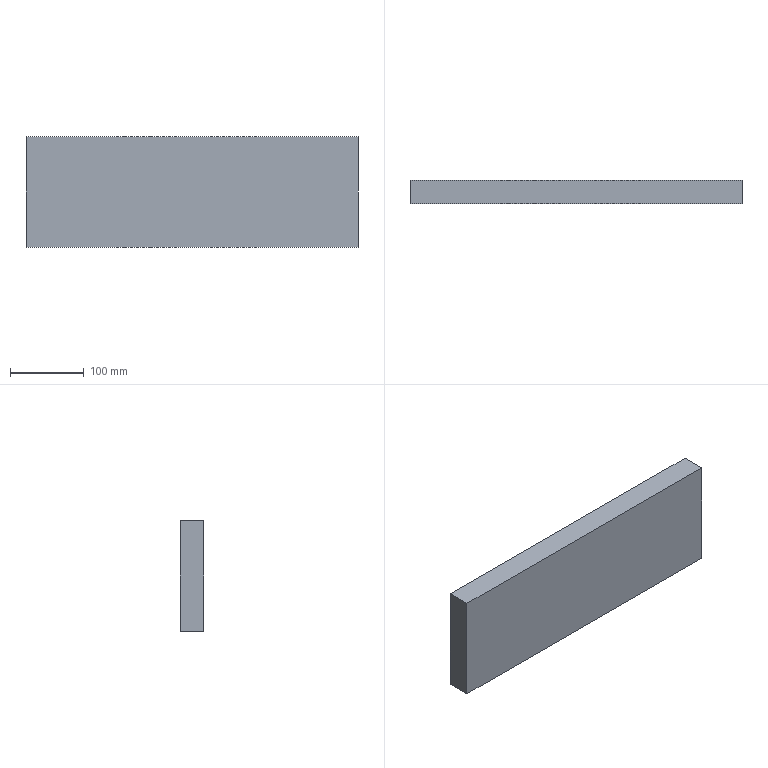Part | NX | 1 solid | 6 faces | box 450 x 32 x 150 mm | volume 2160000 mm3 | plane 6
STEP:
#1=CARTESIAN_POINT('',(225.,0.,75.));
#2=VERTEX_POINT('',#1);
#3=CARTESIAN_POINT('',(225.,0.,-75.));
#4=VERTEX_POINT('',#3);
#5=CARTESIAN_POINT('',(225.,0.,75.));
#6=DIRECTION('',(0.,0.,-1.));
#7=VECTOR('',#6,1000.);
#8=LINE('',#5,#7);
#9=EDGE_CURVE('',#2,#4,#8,.T.);
#10=ORIENTED_EDGE('',*,*,#9,.T.);
#11=CARTESIAN_POINT('',(225.,32.,-75.));
#12=VERTEX_POINT('',#11);
#13=CARTESIAN_POINT('',(225.,32.,-75.));
#14=DIRECTION('',(0.,-1.,0.));
#15=VECTOR('',#14,1000.);
#16=LINE('',#13,#15);
#17=EDGE_CURVE('',#12,#4,#16,.T.);
#18=ORIENTED_EDGE('',*,*,#17,.F.);
#19=CARTESIAN_POINT('',(225.,32.,75.));
#20=VERTEX_POINT('',#19);
#21=CARTESIAN_POINT('',(225.,32.,75.));
#22=DIRECTION('',(0.,0.,-1.));
#23=VECTOR('',#22,1000.);
#24=LINE('',#21,#23);
#25=EDGE_CURVE('',#20,#12,#24,.T.);
#26=ORIENTED_EDGE('',*,*,#25,.F.);
#27=CARTESIAN_POINT('',(225.,32.,75.));
#28=DIRECTION('',(0.,-1.,0.));
#29=VECTOR('',#28,1000.);
#30=LINE('',#27,#29);
#31=EDGE_CURVE('',#20,#2,#30,.T.);
#32=ORIENTED_EDGE('',*,*,#31,.T.);
#33=EDGE_LOOP('',(#10,#18,#26,#32));
#34=FACE_BOUND('',#33,.T.);
#35=CARTESIAN_POINT('',(225.,32.,75.));
#36=DIRECTION('',(-1.,0.,0.));
#37=DIRECTION('',(0.,0.,1.));
#38=AXIS2_PLACEMENT_3D('',#35,#36,#37);
#39=PLANE('',#38);
#40=ADVANCED_FACE('',(#34),#39,.F.);
#41=CARTESIAN_POINT('',(-225.,0.,-75.));
#42=VERTEX_POINT('',#41);
#43=CARTESIAN_POINT('',(-225.,0.,-75.));
#44=DIRECTION('',(-1.,0.,0.));
#45=VECTOR('',#44,1000.);
#46=LINE('',#43,#45);
#47=EDGE_CURVE('',#4,#42,#46,.T.);
#48=ORIENTED_EDGE('',*,*,#47,.T.);
#49=CARTESIAN_POINT('',(-225.,32.,-75.));
#50=VERTEX_POINT('',#49);
#51=CARTESIAN_POINT('',(-225.,32.,-75.));
#52=DIRECTION('',(0.,-1.,0.));
#53=VECTOR('',#52,1000.);
#54=LINE('',#51,#53);
#55=EDGE_CURVE('',#50,#42,#54,.T.);
#56=ORIENTED_EDGE('',*,*,#55,.F.);
#57=CARTESIAN_POINT('',(-225.,32.,-75.));
#58=DIRECTION('',(-1.,0.,0.));
#59=VECTOR('',#58,1000.);
#60=LINE('',#57,#59);
#61=EDGE_CURVE('',#12,#50,#60,.T.);
#62=ORIENTED_EDGE('',*,*,#61,.F.);
#63=ORIENTED_EDGE('',*,*,#17,.T.);
#64=EDGE_LOOP('',(#48,#56,#62,#63));
#65=FACE_BOUND('',#64,.T.);
#66=CARTESIAN_POINT('',(-225.,32.,-75.));
#67=DIRECTION('',(0.,0.,1.));
#68=DIRECTION('',(1.,0.,0.));
#69=AXIS2_PLACEMENT_3D('',#66,#67,#68);
#70=PLANE('',#69);
#71=ADVANCED_FACE('',(#65),#70,.F.);
#72=CARTESIAN_POINT('',(-225.,0.,75.));
#73=VERTEX_POINT('',#72);
#74=CARTESIAN_POINT('',(-225.,0.,75.));
#75=DIRECTION('',(0.,0.,1.));
#76=VECTOR('',#75,1000.);
#77=LINE('',#74,#76);
#78=EDGE_CURVE('',#42,#73,#77,.T.);
#79=ORIENTED_EDGE('',*,*,#78,.T.);
#80=CARTESIAN_POINT('',(-225.,32.,75.));
#81=VERTEX_POINT('',#80);
#82=CARTESIAN_POINT('',(-225.,32.,75.));
#83=DIRECTION('',(0.,-1.,0.));
#84=VECTOR('',#83,1000.);
#85=LINE('',#82,#84);
#86=EDGE_CURVE('',#81,#73,#85,.T.);
#87=ORIENTED_EDGE('',*,*,#86,.F.);
#88=CARTESIAN_POINT('',(-225.,32.,75.));
#89=DIRECTION('',(0.,0.,1.));
#90=VECTOR('',#89,1000.);
#91=LINE('',#88,#90);
#92=EDGE_CURVE('',#50,#81,#91,.T.);
#93=ORIENTED_EDGE('',*,*,#92,.F.);
#94=ORIENTED_EDGE('',*,*,#55,.T.);
#95=EDGE_LOOP('',(#79,#87,#93,#94));
#96=FACE_BOUND('',#95,.T.);
#97=CARTESIAN_POINT('',(-225.,32.,75.));
#98=DIRECTION('',(1.,0.,0.));
#99=DIRECTION('',(0.,0.,-1.));
#100=AXIS2_PLACEMENT_3D('',#97,#98,#99);
#101=PLANE('',#100);
#102=ADVANCED_FACE('',(#96),#101,.F.);
#103=CARTESIAN_POINT('',(-225.,0.,75.));
#104=DIRECTION('',(1.,0.,0.));
#105=VECTOR('',#104,1000.);
#106=LINE('',#103,#105);
#107=EDGE_CURVE('',#73,#2,#106,.T.);
#108=ORIENTED_EDGE('',*,*,#107,.T.);
#109=ORIENTED_EDGE('',*,*,#31,.F.);
#110=CARTESIAN_POINT('',(-225.,32.,75.));
#111=DIRECTION('',(1.,0.,0.));
#112=VECTOR('',#111,1000.);
#113=LINE('',#110,#112);
#114=EDGE_CURVE('',#81,#20,#113,.T.);
#115=ORIENTED_EDGE('',*,*,#114,.F.);
#116=ORIENTED_EDGE('',*,*,#86,.T.);
#117=EDGE_LOOP('',(#108,#109,#115,#116));
#118=FACE_BOUND('',#117,.T.);
#119=CARTESIAN_POINT('',(-225.,32.,75.));
#120=DIRECTION('',(0.,0.,-1.));
#121=DIRECTION('',(-1.,0.,0.));
#122=AXIS2_PLACEMENT_3D('',#119,#120,#121);
#123=PLANE('',#122);
#124=ADVANCED_FACE('',(#118),#123,.F.);
#125=ORIENTED_EDGE('',*,*,#25,.T.);
#126=ORIENTED_EDGE('',*,*,#61,.T.);
#127=ORIENTED_EDGE('',*,*,#92,.T.);
#128=ORIENTED_EDGE('',*,*,#114,.T.);
#129=EDGE_LOOP('',(#125,#126,#127,#128));
#130=FACE_BOUND('',#129,.T.);
#131=CARTESIAN_POINT('',(0.,32.,0.));
#132=DIRECTION('',(0.,-1.,0.));
#133=DIRECTION('',(0.,0.,-1.));
#134=AXIS2_PLACEMENT_3D('',#131,#132,#133);
#135=PLANE('',#134);
#136=ADVANCED_FACE('',(#130),#135,.F.);
#137=ORIENTED_EDGE('',*,*,#9,.F.);
#138=ORIENTED_EDGE('',*,*,#107,.F.);
#139=ORIENTED_EDGE('',*,*,#78,.F.);
#140=ORIENTED_EDGE('',*,*,#47,.F.);
#141=EDGE_LOOP('',(#137,#138,#139,#140));
#142=FACE_BOUND('',#141,.T.);
#143=CARTESIAN_POINT('',(0.,0.,0.));
#144=DIRECTION('',(0.,-1.,0.));
#145=DIRECTION('',(0.,0.,-1.));
#146=AXIS2_PLACEMENT_3D('',#143,#144,#145);
#147=PLANE('',#146);
#148=ADVANCED_FACE('',(#142),#147,.T.);
#149=CLOSED_SHELL('',(#40,#71,#102,#124,#136,#148));
#150=MANIFOLD_SOLID_BREP('',#149);
#151=(LENGTH_UNIT()NAMED_UNIT(*)SI_UNIT(.MILLI.,.METRE.));
#152=UNCERTAINTY_MEASURE_WITH_UNIT(LENGTH_MEASURE(0.00001),#151,'','');
#153=(NAMED_UNIT(*)PLANE_ANGLE_UNIT()SI_UNIT($,.RADIAN.));
#154=(NAMED_UNIT(*)SI_UNIT($,.STERADIAN.)SOLID_ANGLE_UNIT());
#155=(GEOMETRIC_REPRESENTATION_CONTEXT(3)GLOBAL_UNCERTAINTY_ASSIGNED_CONTEXT((#152))GLOBAL_UNIT_ASSIGNED_CONTEXT((#151,#153,#154))REPRESENTATION_CONTEXT('',''));
#156=ADVANCED_BREP_SHAPE_REPRESENTATION('',(#150),#155);